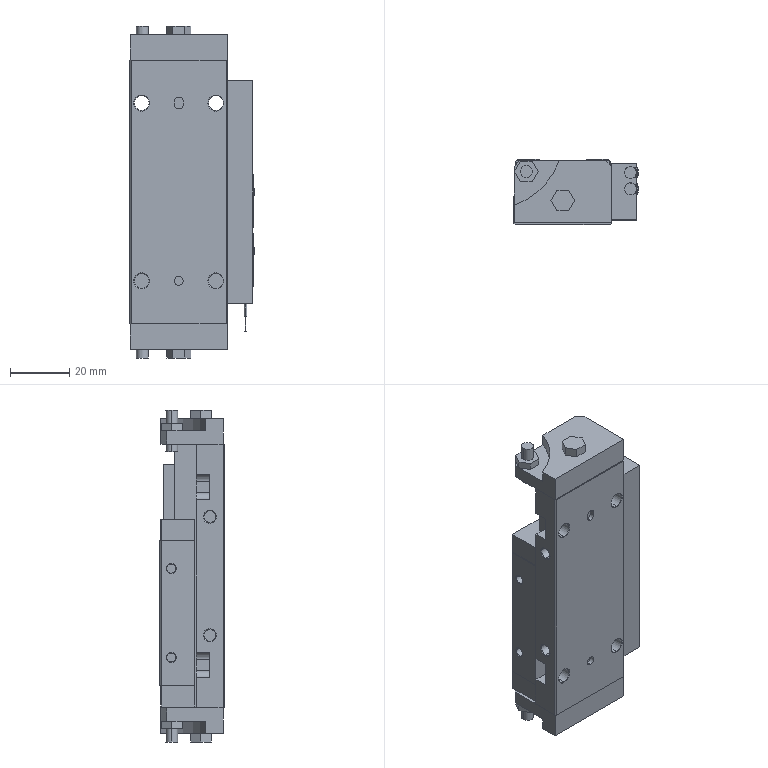Part | NX | 4 solids | 340 faces | box 41.9 x 22 x 112 mm | volume 73904 mm3 | plane 186 | cylinder 106 | cone 48 | commonest cylinder face diameters 4 x32 5 x20 3 x18 0.5 x8 1 x8 2.4 x6